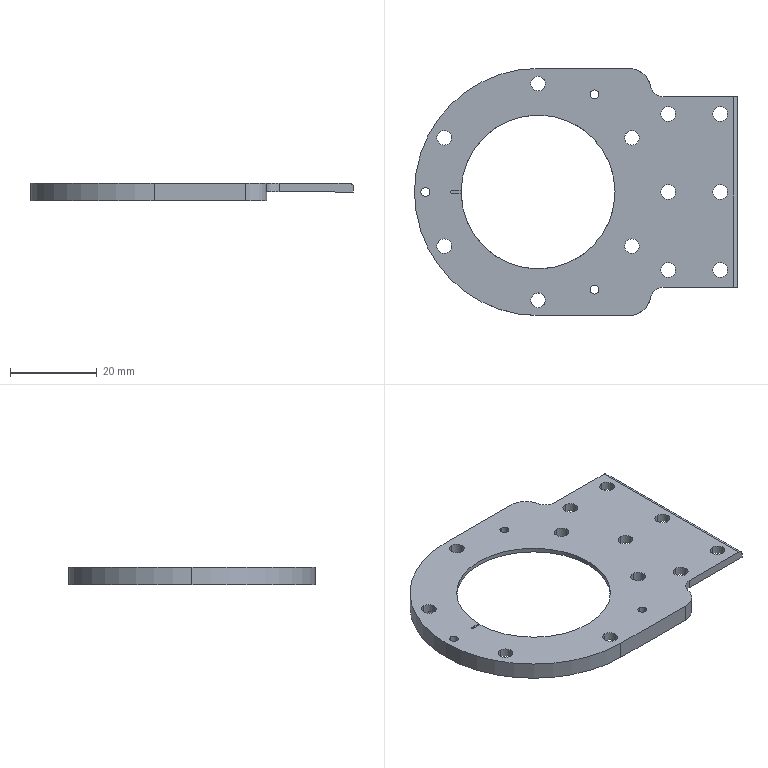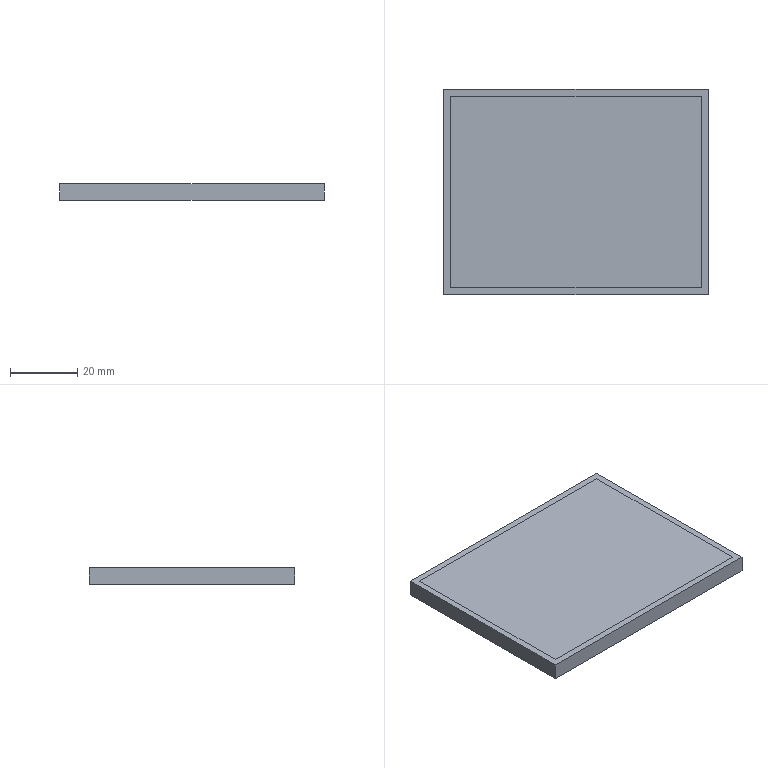CAM job | NX | 3-axis milling, drilling | part box 74.5 x 57 x 4 mm | stock box 78.5 x 61 x 5 mm
Tools:
number,name,description,diameter,corner_radius,flute_length,length,flutes
19,D80,Milling Tool-5 Parameters,80.0,0.0,50.0,75.0,2
1,D6A45,Milling Tool-5 Parameters,6.0,0.0,50.0,75.0,2
17,2.1ZT,Drilling Tool,2.0,0.0,35.0,50.0,2
7,3.4ZT,Drilling Tool,3.4,0.0,35.0,50.0,2
15,D10,Milling Tool-5 Parameters,10.0,0.0,50.0,75.0,2
18,D3R0.5,Milling Tool-5 Parameters,3.0,0.5,50.0,75.0,2
24,D0.5,Milling Tool-5 Parameters,0.5,0.0,50.0,75.0,2
16,D3,Milling Tool-5 Parameters,3.0,0.0,50.0,75.0,2
14,D10JING,Milling Tool-5 Parameters,10.0,0.0,50.0,75.0,2
11,D4,Milling Tool-5 Parameters,4.0,0.0,50.0,75.0,2
Operations:
program,operation,operation_type,tool,method,geometry_group,spindle_rpm,surface_speed,feed_per_tooth,feed_cut,feed_plunge,cut_length_mm,path_length_mm,cut_time_min,machine_time_min
1,FLOOR_WALL,VolumeBased25DMillingOperation,D80,METHOD,A,5000.0,1256.0,0.12,1200.0,100.0,170.5,224.5,0.1421,0.1475
1,SPOT_DRILLING,Operation,D6A45,METHOD,A,9500.0,179.0,0.0132,250.0,0.0,60.0,426.678,0.24,0.2767
1,SPOT_DRILLING_COPY,Operation,2.1ZT,METHOD,A,2500.0,19.0,0.024,120.0,0.0,22.803,201.871,0.19,0.2079
1,SPOT_DRILLING_COPY_COPY,Operation,3.4ZT,METHOD,A,2500.0,19.0,0.024,120.0,0.0,84.258,453.794,0.7021,0.7391
1,ZLEVEL_PROFILE,ZLevelMilling,D10,METHOD,A,9500.0,298.0,0.1842,3500.0,1000.0,1361.699,1422.099,0.4211,0.4272
1,PLANAR_MILL_3,PlanarMilling,D10,METHOD,A,9500.0,298.0,0.1842,3500.0,1000.0,773.038,874.483,0.3702,0.3804
1,ZLEVEL_PROFILE_COPY_1,ZLevelMilling,D3,METHOD,A,9500.0,89.0,0.0632,1200.0,1000.0,270.186,556.941,0.236,0.2647
1,PLANAR_PROFILE,PlanarMilling,D0.5,METHOD,A,9500.0,14.0,0.0368,700.0,50.0,49.711,104.261,0.409,0.4145
1,ZLEVEL_PROFILE_1_COPY_COPY_COPY,ZLevelMilling,D3R0.5,METHOD,A,9500.0,89.0,0.1316,2500.0,1000.0,1092.706,1148.215,0.44,0.4456
1,PLANAR_MILL_2_COPY,PlanarMilling,D6A45,METHOD,A,9500.0,179.0,0.0658,1250.0,100.0,465,1752.336,0.372,0.5007
1,ZLEVEL_PROFILE_COPY_COPY,ZLevelMilling,D10JING,METHOD,A,9500.0,298.0,0.0789,1500.0,1000.0,88.028,154.028,0.06,0.0666
1,ZLEVEL_PROFILE_COPY,ZLevelMilling,D10JING,METHOD,A,9500.0,298.0,0.0632,1200.0,1000.0,1319.642,1385.067,1.1,1.107
2,FLOOR_WALL_COPY,VolumeBased25DMillingOperation,D80,METHOD,B,5000.0,1256.0,0.12,1200.0,100.0,166.5,220.5,0.1388,0.1442
2,FLOOR_WALL_1,VolumeBased25DMillingOperation,D4,METHOD,B,9500.0,119.0,0.1316,2500.0,1000.0,2510.692,2614.979,1.013,1.024
2,FLOOR_WALL_1_COPY,VolumeBased25DMillingOperation,D4,METHOD,B,9500.0,119.0,0.1316,2500.0,700.0,1867.935,1945.881,0.7545,0.7623
2,FLOOR_WALL_1_COPY_COPY,VolumeBased25DMillingOperation,D4,METHOD,B,9500.0,119.0,0.1316,2500.0,700.0,645.288,712.533,0.2625,0.2692
2,FLOOR_WALL_1_COPY_COPY_1,VolumeBased25DMillingOperation,D3,METHOD,B,9500.0,298.0,0.0632,1200.0,700.0,1904.593,2686.51,1.613,1.691
2,PLANAR_MILL_2_COPY_COPY,PlanarMilling,D6A45,METHOD,B,9500.0,179.0,0.0658,1250.0,100.0,393.668,794.224,0.3149,0.355
2,PLANAR_MILL_2_COPY_COPY_COPY,PlanarMilling,D6A45,METHOD,B,9500.0,179.0,0.0658,1250.0,100.0,145.156,674.815,0.1161,0.1691
2,PLANAR_MILL,PlanarMilling,D4,METHOD,B,9500.0,119.0,0.0658,1250.0,100.0,139.182,201.182,0.1113,0.1175